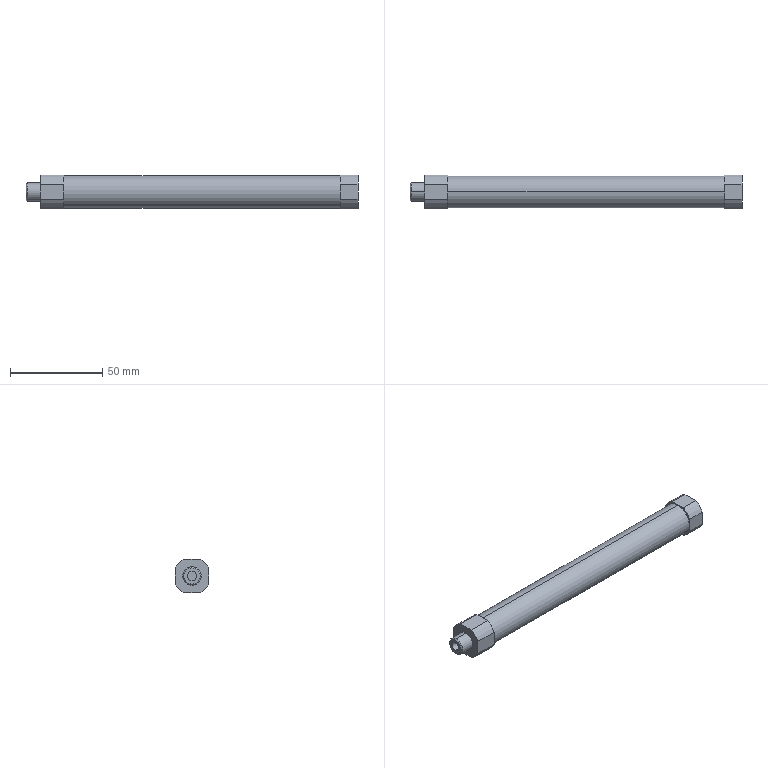Part | SolidWorks | features RefAxis 21, 3DProfileFeature 7, ICE 3, HoleWzd 2, RevCut 1, Revolution 1 | 1 solid | 45 faces | box 180 x 18.3 x 18.3 mm | volume 16108 mm3 | cylinder 20 | plane 15 | cone 10 | commonest cylinder face diameters 20 x8 4.134 x4 5 x2 10 x2 16 x2 17.4 x2
STEP:
#1=CARTESIAN_POINT('',(142.5,0.,-8.));
#2=VERTEX_POINT('',#1);
#3=CARTESIAN_POINT('',(142.5,0.,8.));
#4=VERTEX_POINT('',#3);
#5=CARTESIAN_POINT('',(142.5,0.,0.));
#6=DIRECTION('',(-1.,0.,0.));
#7=DIRECTION('',(0.,0.,1.));
#8=AXIS2_PLACEMENT_3D('',#5,#6,#7);
#9=CIRCLE('',#8,8.);
#10=EDGE_CURVE('',#2,#4,#9,.T.);
#11=ORIENTED_EDGE('',*,*,#10,.F.);
#12=CARTESIAN_POINT('',(12.5,0.,-8.));
#13=VERTEX_POINT('',#12);
#14=CARTESIAN_POINT('',(50.,0.,-8.));
#15=DIRECTION('',(-1.,0.,0.));
#16=VECTOR('',#15,1000.);
#17=LINE('',#14,#16);
#18=EDGE_CURVE('',#2,#13,#17,.T.);
#19=ORIENTED_EDGE('',*,*,#18,.T.);
#20=CARTESIAN_POINT('',(12.5,0.,8.));
#21=VERTEX_POINT('',#20);
#22=CARTESIAN_POINT('',(12.5,0.,0.));
#23=DIRECTION('',(-1.,0.,0.));
#24=DIRECTION('',(0.,0.,1.));
#25=AXIS2_PLACEMENT_3D('',#22,#23,#24);
#26=CIRCLE('',#25,8.);
#27=EDGE_CURVE('',#13,#21,#26,.T.);
#28=ORIENTED_EDGE('',*,*,#27,.T.);
#29=CARTESIAN_POINT('',(50.,0.,8.));
#30=DIRECTION('',(-1.,0.,0.));
#31=VECTOR('',#30,1000.);
#32=LINE('',#29,#31);
#33=EDGE_CURVE('',#4,#21,#32,.T.);
#34=ORIENTED_EDGE('',*,*,#33,.F.);
#35=EDGE_LOOP('',(#11,#19,#28,#34));
#36=FACE_OUTER_BOUND('',#35,.T.);
#37=CARTESIAN_POINT('',(50.,0.,0.));
#38=DIRECTION('',(-1.,0.,0.));
#39=DIRECTION('',(0.,0.,1.));
#40=AXIS2_PLACEMENT_3D('',#37,#38,#39);
#41=CYLINDRICAL_SURFACE('',#40,8.);
#42=ADVANCED_FACE('',(#36),#41,.F.);
#43=CARTESIAN_POINT('',(12.5,0.,-2.5));
#44=VERTEX_POINT('',#43);
#45=CARTESIAN_POINT('',(12.5,0.,2.5));
#46=VERTEX_POINT('',#45);
#47=CARTESIAN_POINT('',(12.5,0.,0.));
#48=DIRECTION('',(-1.,0.,0.));
#49=DIRECTION('',(0.,0.,1.));
#50=AXIS2_PLACEMENT_3D('',#47,#48,#49);
#51=CIRCLE('',#50,2.5);
#52=EDGE_CURVE('',#44,#46,#51,.T.);
#53=ORIENTED_EDGE('',*,*,#52,.F.);
#54=CARTESIAN_POINT('',(-8.,0.,-2.5));
#55=VERTEX_POINT('',#54);
#56=CARTESIAN_POINT('',(50.,0.,-2.5));
#57=DIRECTION('',(-1.,0.,0.));
#58=VECTOR('',#57,1000.);
#59=LINE('',#56,#58);
#60=EDGE_CURVE('',#44,#55,#59,.T.);
#61=ORIENTED_EDGE('',*,*,#60,.T.);
#62=CARTESIAN_POINT('',(-8.,0.,2.5));
#63=VERTEX_POINT('',#62);
#64=CARTESIAN_POINT('',(-8.,0.,0.));
#65=DIRECTION('',(-1.,0.,0.));
#66=DIRECTION('',(0.,0.,1.));
#67=AXIS2_PLACEMENT_3D('',#64,#65,#66);
#68=CIRCLE('',#67,2.5);
#69=EDGE_CURVE('',#55,#63,#68,.T.);
#70=ORIENTED_EDGE('',*,*,#69,.T.);
#71=CARTESIAN_POINT('',(50.,0.,2.5));
#72=DIRECTION('',(-1.,0.,0.));
#73=VECTOR('',#72,1000.);
#74=LINE('',#71,#73);
#75=EDGE_CURVE('',#46,#63,#74,.T.);
#76=ORIENTED_EDGE('',*,*,#75,.F.);
#77=EDGE_LOOP('',(#53,#61,#70,#76));
#78=FACE_OUTER_BOUND('',#77,.T.);
#79=CARTESIAN_POINT('',(50.,0.,0.));
#80=DIRECTION('',(-1.,0.,0.));
#81=DIRECTION('',(0.,0.,1.));
#82=AXIS2_PLACEMENT_3D('',#79,#80,#81);
#83=CYLINDRICAL_SURFACE('',#82,2.5);
#84=ADVANCED_FACE('',(#78),#83,.F.);
#85=CARTESIAN_POINT('',(167.,8.717,-2.067));
#86=VERTEX_POINT('',#85);
#87=CARTESIAN_POINT('',(167.,8.717,2.067));
#88=VERTEX_POINT('',#87);
#89=CARTESIAN_POINT('',(167.,8.717,0.));
#90=DIRECTION('',(0.,1.,0.));
#91=DIRECTION('',(0.,0.,1.));
#92=AXIS2_PLACEMENT_3D('',#89,#90,#91);
#93=CIRCLE('',#92,2.067);
#94=EDGE_CURVE('',#86,#88,#93,.T.);
#95=ORIENTED_EDGE('',*,*,#94,.F.);
#96=CARTESIAN_POINT('',(167.,9.15,-2.5));
#97=VERTEX_POINT('',#96);
#98=CARTESIAN_POINT('',(167.,9.15,-2.5));
#99=DIRECTION('',(0.,0.7071,-0.7071));
#100=VECTOR('',#99,1000.);
#101=LINE('',#98,#100);
#102=EDGE_CURVE('',#86,#97,#101,.T.);
#103=ORIENTED_EDGE('',*,*,#102,.T.);
#104=CARTESIAN_POINT('',(167.,9.15,2.5));
#105=VERTEX_POINT('',#104);
#106=CARTESIAN_POINT('',(167.,9.15,0.));
#107=DIRECTION('',(0.,1.,0.));
#108=DIRECTION('',(0.,0.,1.));
#109=AXIS2_PLACEMENT_3D('',#106,#107,#108);
#110=CIRCLE('',#109,2.5);
#111=EDGE_CURVE('',#97,#105,#110,.T.);
#112=ORIENTED_EDGE('',*,*,#111,.T.);
#113=CARTESIAN_POINT('',(167.,9.15,2.5));
#114=DIRECTION('',(0.,0.7071,0.7071));
#115=VECTOR('',#114,1000.);
#116=LINE('',#113,#115);
#117=EDGE_CURVE('',#88,#105,#116,.T.);
#118=ORIENTED_EDGE('',*,*,#117,.F.);
#119=EDGE_LOOP('',(#95,#103,#112,#118));
#120=FACE_OUTER_BOUND('',#119,.T.);
#121=CARTESIAN_POINT('',(167.,9.15,0.));
#122=DIRECTION('',(0.,1.,0.));
#123=DIRECTION('',(0.,0.,1.));
#124=AXIS2_PLACEMENT_3D('',#121,#122,#123);
#125=CONICAL_SURFACE('',#124,2.5,0.7854);
#126=ADVANCED_FACE('',(#120),#125,.F.);
#127=CARTESIAN_POINT('',(167.,4.15,-2.067));
#128=VERTEX_POINT('',#127);
#129=CARTESIAN_POINT('',(167.,4.15,2.067));
#130=VERTEX_POINT('',#129);
#131=CARTESIAN_POINT('',(167.,4.15,0.));
#132=DIRECTION('',(0.,1.,0.));
#133=DIRECTION('',(0.,0.,1.));
#134=AXIS2_PLACEMENT_3D('',#131,#132,#133);
#135=CIRCLE('',#134,2.067);
#136=EDGE_CURVE('',#128,#130,#135,.T.);
#137=ORIENTED_EDGE('',*,*,#136,.F.);
#138=CARTESIAN_POINT('',(167.,9.15,-2.067));
#139=DIRECTION('',(0.,1.,0.));
#140=VECTOR('',#139,1000.);
#141=LINE('',#138,#140);
#142=EDGE_CURVE('',#128,#86,#141,.T.);
#143=ORIENTED_EDGE('',*,*,#142,.T.);
#144=ORIENTED_EDGE('',*,*,#94,.T.);
#145=CARTESIAN_POINT('',(167.,9.15,2.067));
#146=DIRECTION('',(0.,1.,0.));
#147=VECTOR('',#146,1000.);
#148=LINE('',#145,#147);
#149=EDGE_CURVE('',#130,#88,#148,.T.);
#150=ORIENTED_EDGE('',*,*,#149,.F.);
#151=EDGE_LOOP('',(#137,#143,#144,#150));
#152=FACE_OUTER_BOUND('',#151,.T.);
#153=CARTESIAN_POINT('',(167.,9.15,0.));
#154=DIRECTION('',(0.,1.,0.));
#155=DIRECTION('',(0.,0.,1.));
#156=AXIS2_PLACEMENT_3D('',#153,#154,#155);
#157=CYLINDRICAL_SURFACE('',#156,2.067);
#158=ADVANCED_FACE('',(#152),#157,.F.);
#159=CARTESIAN_POINT('',(167.,2.957,0.));
#160=VERTEX_POINT('',#159);
#161=CARTESIAN_POINT('',(167.,4.15,2.067));
#162=DIRECTION('',(0.,0.5,0.866));
#163=VECTOR('',#162,1000.);
#164=LINE('',#161,#163);
#165=EDGE_CURVE('',#160,#130,#164,.T.);
#166=ORIENTED_EDGE('',*,*,#165,.F.);
#167=CARTESIAN_POINT('',(167.,4.15,-2.067));
#168=DIRECTION('',(0.,0.5,-0.866));
#169=VECTOR('',#168,1000.);
#170=LINE('',#167,#169);
#171=EDGE_CURVE('',#160,#128,#170,.T.);
#172=ORIENTED_EDGE('',*,*,#171,.T.);
#173=ORIENTED_EDGE('',*,*,#136,.T.);
#174=EDGE_LOOP('',(#166,#172,#173));
#175=FACE_OUTER_BOUND('',#174,.T.);
#176=CARTESIAN_POINT('',(167.,4.15,0.));
#177=DIRECTION('',(0.,1.,0.));
#178=DIRECTION('',(0.,0.,1.));
#179=AXIS2_PLACEMENT_3D('',#176,#177,#178);
#180=CONICAL_SURFACE('',#179,2.067,1.047);
#181=ADVANCED_FACE('',(#175),#180,.F.);
#182=CARTESIAN_POINT('',(8.,8.717,-2.067));
#183=VERTEX_POINT('',#182);
#184=CARTESIAN_POINT('',(8.,8.717,2.067));
#185=VERTEX_POINT('',#184);
#186=CARTESIAN_POINT('',(8.,8.717,0.));
#187=DIRECTION('',(0.,1.,0.));
#188=DIRECTION('',(0.,0.,1.));
#189=AXIS2_PLACEMENT_3D('',#186,#187,#188);
#190=CIRCLE('',#189,2.067);
#191=EDGE_CURVE('',#183,#185,#190,.T.);
#192=ORIENTED_EDGE('',*,*,#191,.F.);
#193=CARTESIAN_POINT('',(8.,9.15,-2.5));
#194=VERTEX_POINT('',#193);
#195=CARTESIAN_POINT('',(8.,9.15,-2.5));
#196=DIRECTION('',(0.,0.7071,-0.7071));
#197=VECTOR('',#196,1000.);
#198=LINE('',#195,#197);
#199=EDGE_CURVE('',#183,#194,#198,.T.);
#200=ORIENTED_EDGE('',*,*,#199,.T.);
#201=CARTESIAN_POINT('',(8.,9.15,2.5));
#202=VERTEX_POINT('',#201);
#203=CARTESIAN_POINT('',(8.,9.15,0.));
#204=DIRECTION('',(0.,1.,0.));
#205=DIRECTION('',(0.,0.,1.));
#206=AXIS2_PLACEMENT_3D('',#203,#204,#205);
#207=CIRCLE('',#206,2.5);
#208=EDGE_CURVE('',#194,#202,#207,.T.);
#209=ORIENTED_EDGE('',*,*,#208,.T.);
#210=CARTESIAN_POINT('',(8.,9.15,2.5));
#211=DIRECTION('',(0.,0.7071,0.7071));
#212=VECTOR('',#211,1000.);
#213=LINE('',#210,#212);
#214=EDGE_CURVE('',#185,#202,#213,.T.);
#215=ORIENTED_EDGE('',*,*,#214,.F.);
#216=EDGE_LOOP('',(#192,#200,#209,#215));
#217=FACE_OUTER_BOUND('',#216,.T.);
#218=CARTESIAN_POINT('',(8.,9.15,0.));
#219=DIRECTION('',(0.,1.,0.));
#220=DIRECTION('',(0.,0.,1.));
#221=AXIS2_PLACEMENT_3D('',#218,#219,#220);
#222=CONICAL_SURFACE('',#221,2.5,0.7854);
#223=ADVANCED_FACE('',(#217),#222,.F.);
#224=CARTESIAN_POINT('',(8.,4.15,-2.067));
#225=VERTEX_POINT('',#224);
#226=CARTESIAN_POINT('',(8.,4.15,2.067));
#227=VERTEX_POINT('',#226);
#228=CARTESIAN_POINT('',(8.,4.15,0.));
#229=DIRECTION('',(0.,1.,0.));
#230=DIRECTION('',(0.,0.,1.));
#231=AXIS2_PLACEMENT_3D('',#228,#229,#230);
#232=CIRCLE('',#231,2.067);
#233=EDGE_CURVE('',#225,#227,#232,.T.);
#234=ORIENTED_EDGE('',*,*,#233,.F.);
#235=CARTESIAN_POINT('',(8.,9.15,-2.067));
#236=DIRECTION('',(0.,1.,0.));
#237=VECTOR('',#236,1000.);
#238=LINE('',#235,#237);
#239=EDGE_CURVE('',#225,#183,#238,.T.);
#240=ORIENTED_EDGE('',*,*,#239,.T.);
#241=ORIENTED_EDGE('',*,*,#191,.T.);
#242=CARTESIAN_POINT('',(8.,9.15,2.067));
#243=DIRECTION('',(0.,1.,0.));
#244=VECTOR('',#243,1000.);
#245=LINE('',#242,#244);
#246=EDGE_CURVE('',#227,#185,#245,.T.);
#247=ORIENTED_EDGE('',*,*,#246,.F.);
#248=EDGE_LOOP('',(#234,#240,#241,#247));
#249=FACE_OUTER_BOUND('',#248,.T.);
#250=CARTESIAN_POINT('',(8.,9.15,0.));
#251=DIRECTION('',(0.,1.,0.));
#252=DIRECTION('',(0.,0.,1.));
#253=AXIS2_PLACEMENT_3D('',#250,#251,#252);
#254=CYLINDRICAL_SURFACE('',#253,2.067);
#255=ADVANCED_FACE('',(#249),#254,.F.);
#256=CARTESIAN_POINT('',(8.,2.957,0.));
#257=VERTEX_POINT('',#256);
#258=CARTESIAN_POINT('',(8.,4.15,2.067));
#259=DIRECTION('',(0.,0.5,0.866));
#260=VECTOR('',#259,1000.);
#261=LINE('',#258,#260);
#262=EDGE_CURVE('',#257,#227,#261,.T.);
#263=ORIENTED_EDGE('',*,*,#262,.F.);
#264=CARTESIAN_POINT('',(8.,4.15,-2.067));
#265=DIRECTION('',(0.,0.5,-0.866));
#266=VECTOR('',#265,1000.);
#267=LINE('',#264,#266);
#268=EDGE_CURVE('',#257,#225,#267,.T.);
#269=ORIENTED_EDGE('',*,*,#268,.T.);
#270=ORIENTED_EDGE('',*,*,#233,.T.);
#271=EDGE_LOOP('',(#263,#269,#270));
#272=FACE_OUTER_BOUND('',#271,.T.);
#273=CARTESIAN_POINT('',(8.,4.15,0.));
#274=DIRECTION('',(0.,1.,0.));
#275=DIRECTION('',(0.,0.,1.));
#276=AXIS2_PLACEMENT_3D('',#273,#274,#275);
#277=CONICAL_SURFACE('',#276,2.067,1.047);
#278=ADVANCED_FACE('',(#272),#277,.F.);
#279=CARTESIAN_POINT('',(162.5,0.,-8.7));
#280=VERTEX_POINT('',#279);
#281=CARTESIAN_POINT('',(162.5,0.,8.7));
#282=VERTEX_POINT('',#281);
#283=CARTESIAN_POINT('',(162.5,0.,0.));
#284=DIRECTION('',(1.,0.,0.));
#285=DIRECTION('',(0.,0.,-1.));
#286=AXIS2_PLACEMENT_3D('',#283,#284,#285);
#287=CIRCLE('',#286,8.7);
#288=EDGE_CURVE('',#280,#282,#287,.T.);
#289=ORIENTED_EDGE('',*,*,#288,.F.);
#290=CARTESIAN_POINT('',(12.5,0.,-8.7));
#291=VERTEX_POINT('',#290);
#292=CARTESIAN_POINT('',(162.5,0.,-8.7));
#293=DIRECTION('',(-1.,0.,0.));
#294=VECTOR('',#293,1000.);
#295=LINE('',#292,#294);
#296=EDGE_CURVE('',#280,#291,#295,.T.);
#297=ORIENTED_EDGE('',*,*,#296,.T.);
#298=CARTESIAN_POINT('',(12.5,0.,8.7));
#299=VERTEX_POINT('',#298);
#300=CARTESIAN_POINT('',(12.5,0.,0.));
#301=DIRECTION('',(1.,0.,0.));
#302=DIRECTION('',(0.,0.,-1.));
#303=AXIS2_PLACEMENT_3D('',#300,#301,#302);
#304=CIRCLE('',#303,8.7);
#305=EDGE_CURVE('',#291,#299,#304,.T.);
#306=ORIENTED_EDGE('',*,*,#305,.T.);
#307=CARTESIAN_POINT('',(162.5,0.,8.7));
#308=DIRECTION('',(-1.,0.,0.));
#309=VECTOR('',#308,1000.);
#310=LINE('',#307,#309);
#311=EDGE_CURVE('',#282,#299,#310,.T.);
#312=ORIENTED_EDGE('',*,*,#311,.F.);
#313=EDGE_LOOP('',(#289,#297,#306,#312));
#314=FACE_OUTER_BOUND('',#313,.T.);
#315=CARTESIAN_POINT('',(162.5,0.,0.));
#316=DIRECTION('',(-1.,0.,0.));
#317=DIRECTION('',(0.,0.,1.));
#318=AXIS2_PLACEMENT_3D('',#315,#316,#317);
#319=CYLINDRICAL_SURFACE('',#318,8.7);
#320=ADVANCED_FACE('',(#314),#319,.T.);
#321=CARTESIAN_POINT('',(0.,0.,-5.));
#322=VERTEX_POINT('',#321);
#323=CARTESIAN_POINT('',(0.,0.,5.));
#324=VERTEX_POINT('',#323);
#325=CARTESIAN_POINT('',(0.,0.,0.));
#326=DIRECTION('',(1.,0.,0.));
#327=DIRECTION('',(0.,0.,-1.));
#328=AXIS2_PLACEMENT_3D('',#325,#326,#327);
#329=CIRCLE('',#328,5.);
#330=EDGE_CURVE('',#322,#324,#329,.T.);
#331=ORIENTED_EDGE('',*,*,#330,.F.);
#332=CARTESIAN_POINT('',(-7.386,0.,-5.));
#333=VERTEX_POINT('',#332);
#334=CARTESIAN_POINT('',(0.,0.,-5.));
#335=DIRECTION('',(-1.,0.,0.));
#336=VECTOR('',#335,1000.);
#337=LINE('',#334,#336);
#338=EDGE_CURVE('',#322,#333,#337,.T.);
#339=ORIENTED_EDGE('',*,*,#338,.T.);
#340=CARTESIAN_POINT('',(-7.386,0.,5.));
#341=VERTEX_POINT('',#340);
#342=CARTESIAN_POINT('',(-7.386,0.,0.));
#343=DIRECTION('',(-1.,0.,0.));
#344=DIRECTION('',(0.,0.,1.));
#345=AXIS2_PLACEMENT_3D('',#342,#343,#344);
#346=CIRCLE('',#345,5.);
#347=EDGE_CURVE('',#341,#333,#346,.T.);
#348=ORIENTED_EDGE('',*,*,#347,.F.);
#349=CARTESIAN_POINT('',(0.,0.,5.));
#350=DIRECTION('',(-1.,0.,0.));
#351=VECTOR('',#350,1000.);
#352=LINE('',#349,#351);
#353=EDGE_CURVE('',#324,#341,#352,.T.);
#354=ORIENTED_EDGE('',*,*,#353,.F.);
#355=EDGE_LOOP('',(#331,#339,#348,#354));
#356=FACE_OUTER_BOUND('',#355,.T.);
#357=CARTESIAN_POINT('',(0.,0.,0.));
#358=DIRECTION('',(-1.,0.,0.));
#359=DIRECTION('',(0.,0.,1.));
#360=AXIS2_PLACEMENT_3D('',#357,#358,#359);
#361=CYLINDRICAL_SURFACE('',#360,5.);
#362=ADVANCED_FACE('',(#356),#361,.T.);
#363=CARTESIAN_POINT('',(-8.,0.,4.386));
#364=VERTEX_POINT('',#363);
#365=CARTESIAN_POINT('',(-8.,0.,-4.386));
#366=VERTEX_POINT('',#365);
#367=CARTESIAN_POINT('',(-8.,0.,0.));
#368=DIRECTION('',(-1.,0.,0.));
#369=DIRECTION('',(0.,0.,1.));
#370=AXIS2_PLACEMENT_3D('',#367,#368,#369);
#371=CIRCLE('',#370,4.386);
#372=EDGE_CURVE('',#364,#366,#371,.T.);
#373=ORIENTED_EDGE('',*,*,#372,.F.);
#374=CARTESIAN_POINT('',(-7.386,0.,5.));
#375=DIRECTION('',(0.7071,0.,0.7071));
#376=VECTOR('',#375,1000.);
#377=LINE('',#374,#376);
#378=EDGE_CURVE('',#364,#341,#377,.T.);
#379=ORIENTED_EDGE('',*,*,#378,.T.);
#380=ORIENTED_EDGE('',*,*,#347,.T.);
#381=CARTESIAN_POINT('',(-7.386,0.,-5.));
#382=DIRECTION('',(0.7071,0.,-0.7071));
#383=VECTOR('',#382,1000.);
#384=LINE('',#381,#383);
#385=EDGE_CURVE('',#366,#333,#384,.T.);
#386=ORIENTED_EDGE('',*,*,#385,.F.);
#387=EDGE_LOOP('',(#373,#379,#380,#386));
#388=FACE_OUTER_BOUND('',#387,.T.);
#389=CARTESIAN_POINT('',(-7.386,0.,0.));
#390=DIRECTION('',(1.,0.,0.));
#391=DIRECTION('',(0.,0.,-1.));
#392=AXIS2_PLACEMENT_3D('',#389,#390,#391);
#393=CONICAL_SURFACE('',#392,5.,0.7854);
#394=ADVANCED_FACE('',(#388),#393,.T.);
#395=CARTESIAN_POINT('',(-8.,0.,0.));
#396=DIRECTION('',(-1.,0.,0.));
#397=DIRECTION('',(0.,0.,1.));
#398=AXIS2_PLACEMENT_3D('',#395,#396,#397);
#399=CIRCLE('',#398,4.386);
#400=EDGE_CURVE('',#366,#364,#399,.T.);
#401=ORIENTED_EDGE('',*,*,#400,.T.);
#402=ORIENTED_EDGE('',*,*,#372,.T.);
#403=EDGE_LOOP('',(#401,#402));
#404=FACE_OUTER_BOUND('',#403,.T.);
#405=CARTESIAN_POINT('',(-8.,0.,0.));
#406=DIRECTION('',(-1.,0.,0.));
#407=DIRECTION('',(0.,0.,1.));
#408=AXIS2_PLACEMENT_3D('',#405,#406,#407);
#409=CIRCLE('',#408,2.5);
#410=EDGE_CURVE('',#63,#55,#409,.T.);
#411=ORIENTED_EDGE('',*,*,#410,.F.);
#412=ORIENTED_EDGE('',*,*,#69,.F.);
#413=EDGE_LOOP('',(#411,#412));
#414=FACE_BOUND('',#413,.T.);
#415=CARTESIAN_POINT('',(-8.,0.,0.));
#416=DIRECTION('',(1.,0.,0.));
#417=DIRECTION('',(0.,0.,-1.));
#418=AXIS2_PLACEMENT_3D('',#415,#416,#417);
#419=PLANE('',#418);
#420=ADVANCED_FACE('',(#404,#414),#419,.F.);
#421=CARTESIAN_POINT('',(12.5,-4.035,9.15));
#422=VERTEX_POINT('',#421);
#423=CARTESIAN_POINT('',(12.5,-9.15,4.035));
#424=VERTEX_POINT('',#423);
#425=CARTESIAN_POINT('',(12.5,0.,0.));
#426=DIRECTION('',(1.,0.,0.));
#427=DIRECTION('',(0.,0.,-1.));
#428=AXIS2_PLACEMENT_3D('',#425,#426,#427);
#429=CIRCLE('',#428,10.);
#430=EDGE_CURVE('',#422,#424,#429,.T.);
#431=ORIENTED_EDGE('',*,*,#430,.T.);
#432=CARTESIAN_POINT('',(12.5,-9.15,-4.035));
#433=VERTEX_POINT('',#432);
#434=CARTESIAN_POINT('',(12.5,-9.15,4.035));
#435=DIRECTION('',(0.,0.,-1.));
#436=VECTOR('',#435,1000.);
#437=LINE('',#434,#436);
#438=EDGE_CURVE('',#424,#433,#437,.T.);
#439=ORIENTED_EDGE('',*,*,#438,.T.);
#440=CARTESIAN_POINT('',(12.5,-4.035,-9.15));
#441=VERTEX_POINT('',#440);
#442=CARTESIAN_POINT('',(12.5,0.,0.));
#443=DIRECTION('',(1.,0.,0.));
#444=DIRECTION('',(0.,0.,-1.));
#445=AXIS2_PLACEMENT_3D('',#442,#443,#444);
#446=CIRCLE('',#445,10.);
#447=EDGE_CURVE('',#433,#441,#446,.T.);
#448=ORIENTED_EDGE('',*,*,#447,.T.);
#449=CARTESIAN_POINT('',(12.5,4.035,-9.15));
#450=VERTEX_POINT('',#449);
#451=CARTESIAN_POINT('',(12.5,-4.035,-9.15));
#452=DIRECTION('',(0.,1.,0.));
#453=VECTOR('',#452,1000.);
#454=LINE('',#451,#453);
#455=EDGE_CURVE('',#441,#450,#454,.T.);
#456=ORIENTED_EDGE('',*,*,#455,.T.);
#457=CARTESIAN_POINT('',(12.5,9.15,-4.035));
#458=VERTEX_POINT('',#457);
#459=CARTESIAN_POINT('',(12.5,0.,0.));
#460=DIRECTION('',(1.,0.,0.));
#461=DIRECTION('',(0.,0.,-1.));
#462=AXIS2_PLACEMENT_3D('',#459,#460,#461);
#463=CIRCLE('',#462,10.);
#464=EDGE_CURVE('',#450,#458,#463,.T.);
#465=ORIENTED_EDGE('',*,*,#464,.T.);
#466=CARTESIAN_POINT('',(12.5,9.15,4.035));
#467=VERTEX_POINT('',#466);
#468=CARTESIAN_POINT('',(12.5,9.15,-4.035));
#469=DIRECTION('',(0.,0.,1.));
#470=VECTOR('',#469,1000.);
#471=LINE('',#468,#470);
#472=EDGE_CURVE('',#458,#467,#471,.T.);
#473=ORIENTED_EDGE('',*,*,#472,.T.);
#474=CARTESIAN_POINT('',(12.5,4.035,9.15));
#475=VERTEX_POINT('',#474);
#476=CARTESIAN_POINT('',(12.5,0.,0.));
#477=DIRECTION('',(1.,0.,0.));
#478=DIRECTION('',(0.,0.,-1.));
#479=AXIS2_PLACEMENT_3D('',#476,#477,#478);
#480=CIRCLE('',#479,10.);
#481=EDGE_CURVE('',#467,#475,#480,.T.);
#482=ORIENTED_EDGE('',*,*,#481,.T.);
#483=CARTESIAN_POINT('',(12.5,4.035,9.15));
#484=DIRECTION('',(0.,-1.,0.));
#485=VECTOR('',#484,1000.);
#486=LINE('',#483,#485);
#487=EDGE_CURVE('',#475,#422,#486,.T.);
#488=ORIENTED_EDGE('',*,*,#487,.T.);
#489=EDGE_LOOP('',(#431,#439,#448,#456,#465,#473,#482,#488));
#490=FACE_OUTER_BOUND('',#489,.T.);
#491=CARTESIAN_POINT('',(12.5,0.,0.));
#492=DIRECTION('',(1.,0.,0.));
#493=DIRECTION('',(0.,0.,-1.));
#494=AXIS2_PLACEMENT_3D('',#491,#492,#493);
#495=CIRCLE('',#494,8.7);
#496=EDGE_CURVE('',#299,#291,#495,.T.);
#497=ORIENTED_EDGE('',*,*,#496,.F.);
#498=ORIENTED_EDGE('',*,*,#305,.F.);
#499=EDGE_LOOP('',(#497,#498));
#500=FACE_BOUND('',#499,.T.);
#501=CARTESIAN_POINT('',(12.5,0.,0.));
#502=DIRECTION('',(1.,0.,0.));
#503=DIRECTION('',(0.,0.,-1.));
#504=AXIS2_PLACEMENT_3D('',#501,#502,#503);
#505=PLANE('',#504);
#506=ADVANCED_FACE('',(#490,#500),#505,.T.);
#507=ORIENTED_EDGE('',*,*,#378,.F.);
#508=ORIENTED_EDGE('',*,*,#400,.F.);
#509=ORIENTED_EDGE('',*,*,#385,.T.);
#510=CARTESIAN_POINT('',(-7.386,0.,0.));
#511=DIRECTION('',(-1.,0.,0.));
#512=DIRECTION('',(0.,0.,1.));
#513=AXIS2_PLACEMENT_3D('',#510,#511,#512);
#514=CIRCLE('',#513,5.);
#515=EDGE_CURVE('',#333,#341,#514,.T.);
#516=ORIENTED_EDGE('',*,*,#515,.T.);
#517=EDGE_LOOP('',(#507,#508,#509,#516));
#518=FACE_OUTER_BOUND('',#517,.T.);
#519=CARTESIAN_POINT('',(-7.386,0.,0.));
#520=DIRECTION('',(1.,0.,0.));
#521=DIRECTION('',(0.,0.,-1.));
#522=AXIS2_PLACEMENT_3D('',#519,#520,#521);
#523=CONICAL_SURFACE('',#522,5.,0.7854);
#524=ADVANCED_FACE('',(#518),#523,.T.);
#525=ORIENTED_EDGE('',*,*,#338,.F.);
#526=CARTESIAN_POINT('',(0.,0.,0.));
#527=DIRECTION('',(1.,0.,0.));
#528=DIRECTION('',(0.,0.,-1.));
#529=AXIS2_PLACEMENT_3D('',#526,#527,#528);
#530=CIRCLE('',#529,5.);
#531=EDGE_CURVE('',#324,#322,#530,.T.);
#532=ORIENTED_EDGE('',*,*,#531,.F.);
#533=ORIENTED_EDGE('',*,*,#353,.T.);
#534=ORIENTED_EDGE('',*,*,#515,.F.);
#535=EDGE_LOOP('',(#525,#532,#533,#534));
#536=FACE_OUTER_BOUND('',#535,.T.);
#537=CARTESIAN_POINT('',(0.,0.,0.));
#538=DIRECTION('',(-1.,0.,0.));
#539=DIRECTION('',(0.,0.,1.));
#540=AXIS2_PLACEMENT_3D('',#537,#538,#539);
#541=CYLINDRICAL_SURFACE('',#540,5.);
#542=ADVANCED_FACE('',(#536),#541,.T.);
#543=CARTESIAN_POINT('',(0.,-4.035,9.15));
#544=VERTEX_POINT('',#543);
#545=CARTESIAN_POINT('',(0.,-9.15,4.035));
#546=VERTEX_POINT('',#545);
#547=CARTESIAN_POINT('',(0.,0.,0.));
#548=DIRECTION('',(1.,0.,0.));
#549=DIRECTION('',(0.,0.,-1.));
#550=AXIS2_PLACEMENT_3D('',#547,#548,#549);
#551=CIRCLE('',#550,10.);
#552=EDGE_CURVE('',#544,#546,#551,.T.);
#553=ORIENTED_EDGE('',*,*,#552,.F.);
#554=CARTESIAN_POINT('',(0.,4.035,9.15));
#555=VERTEX_POINT('',#554);
#556=CARTESIAN_POINT('',(0.,4.035,9.15));
#557=DIRECTION('',(0.,-1.,0.));
#558=VECTOR('',#557,1000.);
#559=LINE('',#556,#558);
#560=EDGE_CURVE('',#555,#544,#559,.T.);
#561=ORIENTED_EDGE('',*,*,#560,.F.);
#562=CARTESIAN_POINT('',(0.,9.15,4.035));
#563=VERTEX_POINT('',#562);
#564=CARTESIAN_POINT('',(0.,0.,0.));
#565=DIRECTION('',(1.,0.,0.));
#566=DIRECTION('',(0.,0.,-1.));
#567=AXIS2_PLACEMENT_3D('',#564,#565,#566);
#568=CIRCLE('',#567,10.);
#569=EDGE_CURVE('',#563,#555,#568,.T.);
#570=ORIENTED_EDGE('',*,*,#569,.F.);
#571=CARTESIAN_POINT('',(0.,9.15,-4.035));
#572=VERTEX_POINT('',#571);
#573=CARTESIAN_POINT('',(0.,9.15,-4.035));
#574=DIRECTION('',(0.,0.,1.));
#575=VECTOR('',#574,1000.);
#576=LINE('',#573,#575);
#577=EDGE_CURVE('',#572,#563,#576,.T.);
#578=ORIENTED_EDGE('',*,*,#577,.F.);
#579=CARTESIAN_POINT('',(0.,4.035,-9.15));
#580=VERTEX_POINT('',#579);
#581=CARTESIAN_POINT('',(0.,0.,0.));
#582=DIRECTION('',(1.,0.,0.));
#583=DIRECTION('',(0.,0.,-1.));
#584=AXIS2_PLACEMENT_3D('',#581,#582,#583);
#585=CIRCLE('',#584,10.);
#586=EDGE_CURVE('',#580,#572,#585,.T.);
#587=ORIENTED_EDGE('',*,*,#586,.F.);
#588=CARTESIAN_POINT('',(0.,-4.035,-9.15));
#589=VERTEX_POINT('',#588);
#590=CARTESIAN_POINT('',(0.,-4.035,-9.15));
#591=DIRECTION('',(0.,1.,0.));
#592=VECTOR('',#591,1000.);
#593=LINE('',#590,#592);
#594=EDGE_CURVE('',#589,#580,#593,.T.);
#595=ORIENTED_EDGE('',*,*,#594,.F.);
#596=CARTESIAN_POINT('',(0.,-9.15,-4.035));
#597=VERTEX_POINT('',#596);
#598=CARTESIAN_POINT('',(0.,0.,0.));
#599=DIRECTION('',(1.,0.,0.));
#600=DIRECTION('',(0.,0.,-1.));
#601=AXIS2_PLACEMENT_3D('',#598,#599,#600);
#602=CIRCLE('',#601,10.);
#603=EDGE_CURVE('',#597,#589,#602,.T.);
#604=ORIENTED_EDGE('',*,*,#603,.F.);
#605=CARTESIAN_POINT('',(0.,-9.15,4.035));
#606=DIRECTION('',(0.,0.,-1.));
#607=VECTOR('',#606,1000.);
#608=LINE('',#605,#607);
#609=EDGE_CURVE('',#546,#597,#608,.T.);
#610=ORIENTED_EDGE('',*,*,#609,.F.);
#611=EDGE_LOOP('',(#553,#561,#570,#578,#587,#595,#604,#610));
#612=FACE_OUTER_BOUND('',#611,.T.);
#613=ORIENTED_EDGE('',*,*,#531,.T.);
#614=ORIENTED_EDGE('',*,*,#330,.T.);
#615=EDGE_LOOP('',(#613,#614));
#616=FACE_BOUND('',#615,.T.);
#617=CARTESIAN_POINT('',(0.,0.,0.));
#618=DIRECTION('',(1.,0.,0.));
#619=DIRECTION('',(0.,0.,-1.));
#620=AXIS2_PLACEMENT_3D('',#617,#618,#619);
#621=PLANE('',#620);
#622=ADVANCED_FACE('',(#612,#616),#621,.F.);
#623=ORIENTED_EDGE('',*,*,#552,.T.);
#624=CARTESIAN_POINT('',(12.5,-9.15,4.035));
#625=DIRECTION('',(-1.,0.,0.));
#626=VECTOR('',#625,1000.);
#627=LINE('',#624,#626);
#628=EDGE_CURVE('',#424,#546,#627,.T.);
#629=ORIENTED_EDGE('',*,*,#628,.F.);
#630=ORIENTED_EDGE('',*,*,#430,.F.);
#631=CARTESIAN_POINT('',(12.5,-4.035,9.15));
#632=DIRECTION('',(-1.,0.,0.));
#633=VECTOR('',#632,1000.);
#634=LINE('',#631,#633);
#635=EDGE_CURVE('',#422,#544,#634,.T.);
#636=ORIENTED_EDGE('',*,*,#635,.T.);
#637=EDGE_LOOP('',(#623,#629,#630,#636));
#638=FACE_OUTER_BOUND('',#637,.T.);
#639=CARTESIAN_POINT('',(12.5,0.,0.));
#640=DIRECTION('',(-1.,0.,0.));
#641=DIRECTION('',(0.,0.,1.));
#642=AXIS2_PLACEMENT_3D('',#639,#640,#641);
#643=CYLINDRICAL_SURFACE('',#642,10.);
#644=ADVANCED_FACE('',(#638),#643,.T.);
#645=ORIENTED_EDGE('',*,*,#609,.T.);
#646=CARTESIAN_POINT('',(12.5,-9.15,-4.035));
#647=DIRECTION('',(-1.,0.,0.));
#648=VECTOR('',#647,1000.);
#649=LINE('',#646,#648);
#650=EDGE_CURVE('',#433,#597,#649,.T.);
#651=ORIENTED_EDGE('',*,*,#650,.F.);
#652=ORIENTED_EDGE('',*,*,#438,.F.);
#653=ORIENTED_EDGE('',*,*,#628,.T.);
#654=EDGE_LOOP('',(#645,#651,#652,#653));
#655=FACE_OUTER_BOUND('',#654,.T.);
#656=CARTESIAN_POINT('',(12.5,-9.15,4.035));
#657=DIRECTION('',(0.,1.,0.));
#658=DIRECTION('',(0.,0.,1.));
#659=AXIS2_PLACEMENT_3D('',#656,#657,#658);
#660=PLANE('',#659);
#661=ADVANCED_FACE('',(#655),#660,.F.);
#662=ORIENTED_EDGE('',*,*,#603,.T.);
#663=CARTESIAN_POINT('',(12.5,-4.035,-9.15));
#664=DIRECTION('',(-1.,0.,0.));
#665=VECTOR('',#664,1000.);
#666=LINE('',#663,#665);
#667=EDGE_CURVE('',#441,#589,#666,.T.);
#668=ORIENTED_EDGE('',*,*,#667,.F.);
#669=ORIENTED_EDGE('',*,*,#447,.F.);
#670=ORIENTED_EDGE('',*,*,#650,.T.);
#671=EDGE_LOOP('',(#662,#668,#669,#670));
#672=FACE_OUTER_BOUND('',#671,.T.);
#673=CARTESIAN_POINT('',(12.5,0.,0.));
#674=DIRECTION('',(-1.,0.,0.));
#675=DIRECTION('',(0.,0.,1.));
#676=AXIS2_PLACEMENT_3D('',#673,#674,#675);
#677=CYLINDRICAL_SURFACE('',#676,10.);
#678=ADVANCED_FACE('',(#672),#677,.T.);
#679=ORIENTED_EDGE('',*,*,#594,.T.);
#680=CARTESIAN_POINT('',(12.5,4.035,-9.15));
#681=DIRECTION('',(-1.,0.,0.));
#682=VECTOR('',#681,1000.);
#683=LINE('',#680,#682);
#684=EDGE_CURVE('',#450,#580,#683,.T.);
#685=ORIENTED_EDGE('',*,*,#684,.F.);
#686=ORIENTED_EDGE('',*,*,#455,.F.);
#687=ORIENTED_EDGE('',*,*,#667,.T.);
#688=EDGE_LOOP('',(#679,#685,#686,#687));
#689=FACE_OUTER_BOUND('',#688,.T.);
#690=CARTESIAN_POINT('',(12.5,-4.035,-9.15));
#691=DIRECTION('',(0.,0.,1.));
#692=DIRECTION('',(1.,0.,0.));
#693=AXIS2_PLACEMENT_3D('',#690,#691,#692);
#694=PLANE('',#693);
#695=ADVANCED_FACE('',(#689),#694,.F.);
#696=ORIENTED_EDGE('',*,*,#586,.T.);
#697=CARTESIAN_POINT('',(12.5,9.15,-4.035));
#698=DIRECTION('',(-1.,0.,0.));
#699=VECTOR('',#698,1000.);
#700=LINE('',#697,#699);
#701=EDGE_CURVE('',#458,#572,#700,.T.);
#702=ORIENTED_EDGE('',*,*,#701,.F.);
#703=ORIENTED_EDGE('',*,*,#464,.F.);
#704=ORIENTED_EDGE('',*,*,#684,.T.);
#705=EDGE_LOOP('',(#696,#702,#703,#704));
#706=FACE_OUTER_BOUND('',#705,.T.);
#707=CARTESIAN_POINT('',(12.5,0.,0.));
#708=DIRECTION('',(-1.,0.,0.));
#709=DIRECTION('',(0.,0.,1.));
#710=AXIS2_PLACEMENT_3D('',#707,#708,#709);
#711=CYLINDRICAL_SURFACE('',#710,10.);
#712=ADVANCED_FACE('',(#706),#711,.T.);
#713=CARTESIAN_POINT('',(8.,9.15,0.));
#714=DIRECTION('',(0.,1.,0.));
#715=DIRECTION('',(0.,0.,1.));
#716=AXIS2_PLACEMENT_3D('',#713,#714,#715);
#717=CIRCLE('',#716,2.5);
#718=EDGE_CURVE('',#202,#194,#717,.T.);
#719=ORIENTED_EDGE('',*,*,#718,.F.);
#720=ORIENTED_EDGE('',*,*,#208,.F.);
#721=EDGE_LOOP('',(#719,#720));
#722=FACE_BOUND('',#721,.T.);
#723=ORIENTED_EDGE('',*,*,#577,.T.);
#724=CARTESIAN_POINT('',(12.5,9.15,4.035));
#725=DIRECTION('',(-1.,0.,0.));
#726=VECTOR('',#725,1000.);
#727=LINE('',#724,#726);
#728=EDGE_CURVE('',#467,#563,#727,.T.);
#729=ORIENTED_EDGE('',*,*,#728,.F.);
#730=ORIENTED_EDGE('',*,*,#472,.F.);
#731=ORIENTED_EDGE('',*,*,#701,.T.);
#732=EDGE_LOOP('',(#723,#729,#730,#731));
#733=FACE_OUTER_BOUND('',#732,.T.);
#734=CARTESIAN_POINT('',(12.5,9.15,-4.035));
#735=DIRECTION('',(0.,-1.,0.));
#736=DIRECTION('',(0.,0.,-1.));
#737=AXIS2_PLACEMENT_3D('',#734,#735,#736);
#738=PLANE('',#737);
#739=ADVANCED_FACE('',(#722,#733),#738,.F.);
#740=ORIENTED_EDGE('',*,*,#569,.T.);
#741=CARTESIAN_POINT('',(12.5,4.035,9.15));
#742=DIRECTION('',(-1.,0.,0.));
#743=VECTOR('',#742,1000.);
#744=LINE('',#741,#743);
#745=EDGE_CURVE('',#475,#555,#744,.T.);
#746=ORIENTED_EDGE('',*,*,#745,.F.);
#747=ORIENTED_EDGE('',*,*,#481,.F.);
#748=ORIENTED_EDGE('',*,*,#728,.T.);
#749=EDGE_LOOP('',(#740,#746,#747,#748));
#750=FACE_OUTER_BOUND('',#749,.T.);
#751=CARTESIAN_POINT('',(12.5,0.,0.));
#752=DIRECTION('',(-1.,0.,0.));
#753=DIRECTION('',(0.,0.,1.));
#754=AXIS2_PLACEMENT_3D('',#751,#752,#753);
#755=CYLINDRICAL_SURFACE('',#754,10.);
#756=ADVANCED_FACE('',(#750),#755,.T.);
#757=ORIENTED_EDGE('',*,*,#560,.T.);
#758=ORIENTED_EDGE('',*,*,#635,.F.);
#759=ORIENTED_EDGE('',*,*,#487,.F.);
#760=ORIENTED_EDGE('',*,*,#745,.T.);
#761=EDGE_LOOP('',(#757,#758,#759,#760));
#762=FACE_OUTER_BOUND('',#761,.T.);
#763=CARTESIAN_POINT('',(12.5,4.035,9.15));
#764=DIRECTION('',(0.,0.,-1.));
#765=DIRECTION('',(-1.,0.,0.));
#766=AXIS2_PLACEMENT_3D('',#763,#764,#765);
#767=PLANE('',#766);
#768=ADVANCED_FACE('',(#762),#767,.F.);
#769=ORIENTED_EDGE('',*,*,#296,.F.);
#770=CARTESIAN_POINT('',(162.5,0.,0.));
#771=DIRECTION('',(1.,0.,0.));
#772=DIRECTION('',(0.,0.,-1.));
#773=AXIS2_PLACEMENT_3D('',#770,#771,#772);
#774=CIRCLE('',#773,8.7);
#775=EDGE_CURVE('',#282,#280,#774,.T.);
#776=ORIENTED_EDGE('',*,*,#775,.F.);
#777=ORIENTED_EDGE('',*,*,#311,.T.);
#778=ORIENTED_EDGE('',*,*,#496,.T.);
#779=EDGE_LOOP('',(#769,#776,#777,#778));
#780=FACE_OUTER_BOUND('',#779,.T.);
#781=CARTESIAN_POINT('',(162.5,0.,0.));
#782=DIRECTION('',(-1.,0.,0.));
#783=DIRECTION('',(0.,0.,1.));
#784=AXIS2_PLACEMENT_3D('',#781,#782,#783);
#785=CYLINDRICAL_SURFACE('',#784,8.7);
#786=ADVANCED_FACE('',(#780),#785,.T.);
#787=CARTESIAN_POINT('',(162.5,-4.035,9.15));
#788=VERTEX_POINT('',#787);
#789=CARTESIAN_POINT('',(162.5,-9.15,4.035));
#790=VERTEX_POINT('',#789);
#791=CARTESIAN_POINT('',(162.5,0.,0.));
#792=DIRECTION('',(1.,0.,0.));
#793=DIRECTION('',(0.,0.,-1.));
#794=AXIS2_PLACEMENT_3D('',#791,#792,#793);
#795=CIRCLE('',#794,10.);
#796=EDGE_CURVE('',#788,#790,#795,.T.);
#797=ORIENTED_EDGE('',*,*,#796,.F.);
#798=CARTESIAN_POINT('',(162.5,4.035,9.15));
#799=VERTEX_POINT('',#798);
#800=CARTESIAN_POINT('',(162.5,4.035,9.15));
#801=DIRECTION('',(0.,-1.,0.));
#802=VECTOR('',#801,1000.);
#803=LINE('',#800,#802);
#804=EDGE_CURVE('',#799,#788,#803,.T.);
#805=ORIENTED_EDGE('',*,*,#804,.F.);
#806=CARTESIAN_POINT('',(162.5,9.15,4.035));
#807=VERTEX_POINT('',#806);
#808=CARTESIAN_POINT('',(162.5,0.,0.));
#809=DIRECTION('',(1.,0.,0.));
#810=DIRECTION('',(0.,0.,-1.));
#811=AXIS2_PLACEMENT_3D('',#808,#809,#810);
#812=CIRCLE('',#811,10.);
#813=EDGE_CURVE('',#807,#799,#812,.T.);
#814=ORIENTED_EDGE('',*,*,#813,.F.);
#815=CARTESIAN_POINT('',(162.5,9.15,-4.035));
#816=VERTEX_POINT('',#815);
#817=CARTESIAN_POINT('',(162.5,9.15,-4.035));
#818=DIRECTION('',(0.,0.,1.));
#819=VECTOR('',#818,1000.);
#820=LINE('',#817,#819);
#821=EDGE_CURVE('',#816,#807,#820,.T.);
#822=ORIENTED_EDGE('',*,*,#821,.F.);
#823=CARTESIAN_POINT('',(162.5,4.035,-9.15));
#824=VERTEX_POINT('',#823);
#825=CARTESIAN_POINT('',(162.5,0.,0.));
#826=DIRECTION('',(1.,0.,0.));
#827=DIRECTION('',(0.,0.,-1.));
#828=AXIS2_PLACEMENT_3D('',#825,#826,#827);
#829=CIRCLE('',#828,10.);
#830=EDGE_CURVE('',#824,#816,#829,.T.);
#831=ORIENTED_EDGE('',*,*,#830,.F.);
#832=CARTESIAN_POINT('',(162.5,-4.035,-9.15));
#833=VERTEX_POINT('',#832);
#834=CARTESIAN_POINT('',(162.5,-4.035,-9.15));
#835=DIRECTION('',(0.,1.,0.));
#836=VECTOR('',#835,1000.);
#837=LINE('',#834,#836);
#838=EDGE_CURVE('',#833,#824,#837,.T.);
#839=ORIENTED_EDGE('',*,*,#838,.F.);
#840=CARTESIAN_POINT('',(162.5,-9.15,-4.035));
#841=VERTEX_POINT('',#840);
#842=CARTESIAN_POINT('',(162.5,0.,0.));
#843=DIRECTION('',(1.,0.,0.));
#844=DIRECTION('',(0.,0.,-1.));
#845=AXIS2_PLACEMENT_3D('',#842,#843,#844);
#846=CIRCLE('',#845,10.);
#847=EDGE_CURVE('',#841,#833,#846,.T.);
#848=ORIENTED_EDGE('',*,*,#847,.F.);
#849=CARTESIAN_POINT('',(162.5,-9.15,4.035));
#850=DIRECTION('',(0.,0.,-1.));
#851=VECTOR('',#850,1000.);
#852=LINE('',#849,#851);
#853=EDGE_CURVE('',#790,#841,#852,.T.);
#854=ORIENTED_EDGE('',*,*,#853,.F.);
#855=EDGE_LOOP('',(#797,#805,#814,#822,#831,#839,#848,#854));
#856=FACE_OUTER_BOUND('',#855,.T.);
#857=ORIENTED_EDGE('',*,*,#775,.T.);
#858=ORIENTED_EDGE('',*,*,#288,.T.);
#859=EDGE_LOOP('',(#857,#858));
#860=FACE_BOUND('',#859,.T.);
#861=CARTESIAN_POINT('',(162.5,0.,0.));
#862=DIRECTION('',(1.,0.,0.));
#863=DIRECTION('',(0.,0.,-1.));
#864=AXIS2_PLACEMENT_3D('',#861,#862,#863);
#865=PLANE('',#864);
#866=ADVANCED_FACE('',(#856,#860),#865,.F.);
#867=ORIENTED_EDGE('',*,*,#796,.T.);
#868=CARTESIAN_POINT('',(172.,-9.15,4.035));
#869=VERTEX_POINT('',#868);
#870=CARTESIAN_POINT('',(172.,-9.15,4.035));
#871=DIRECTION('',(-1.,0.,0.));
#872=VECTOR('',#871,1000.);
#873=LINE('',#870,#872);
#874=EDGE_CURVE('',#869,#790,#873,.T.);
#875=ORIENTED_EDGE('',*,*,#874,.F.);
#876=CARTESIAN_POINT('',(172.,-4.035,9.15));
#877=VERTEX_POINT('',#876);
#878=CARTESIAN_POINT('',(172.,0.,0.));
#879=DIRECTION('',(1.,0.,0.));
#880=DIRECTION('',(0.,0.,-1.));
#881=AXIS2_PLACEMENT_3D('',#878,#879,#880);
#882=CIRCLE('',#881,10.);
#883=EDGE_CURVE('',#877,#869,#882,.T.);
#884=ORIENTED_EDGE('',*,*,#883,.F.);
#885=CARTESIAN_POINT('',(172.,-4.035,9.15));
#886=DIRECTION('',(-1.,0.,0.));
#887=VECTOR('',#886,1000.);
#888=LINE('',#885,#887);
#889=EDGE_CURVE('',#877,#788,#888,.T.);
#890=ORIENTED_EDGE('',*,*,#889,.T.);
#891=EDGE_LOOP('',(#867,#875,#884,#890));
#892=FACE_OUTER_BOUND('',#891,.T.);
#893=CARTESIAN_POINT('',(172.,0.,0.));
#894=DIRECTION('',(-1.,0.,0.));
#895=DIRECTION('',(0.,0.,1.));
#896=AXIS2_PLACEMENT_3D('',#893,#894,#895);
#897=CYLINDRICAL_SURFACE('',#896,10.);
#898=ADVANCED_FACE('',(#892),#897,.T.);
#899=ORIENTED_EDGE('',*,*,#853,.T.);
#900=CARTESIAN_POINT('',(172.,-9.15,-4.035));
#901=VERTEX_POINT('',#900);
#902=CARTESIAN_POINT('',(172.,-9.15,-4.035));
#903=DIRECTION('',(-1.,0.,0.));
#904=VECTOR('',#903,1000.);
#905=LINE('',#902,#904);
#906=EDGE_CURVE('',#901,#841,#905,.T.);
#907=ORIENTED_EDGE('',*,*,#906,.F.);
#908=CARTESIAN_POINT('',(172.,-9.15,4.035));
#909=DIRECTION('',(0.,0.,-1.));
#910=VECTOR('',#909,1000.);
#911=LINE('',#908,#910);
#912=EDGE_CURVE('',#869,#901,#911,.T.);
#913=ORIENTED_EDGE('',*,*,#912,.F.);
#914=ORIENTED_EDGE('',*,*,#874,.T.);
#915=EDGE_LOOP('',(#899,#907,#913,#914));
#916=FACE_OUTER_BOUND('',#915,.T.);
#917=CARTESIAN_POINT('',(172.,-9.15,4.035));
#918=DIRECTION('',(0.,1.,0.));
#919=DIRECTION('',(0.,0.,1.));
#920=AXIS2_PLACEMENT_3D('',#917,#918,#919);
#921=PLANE('',#920);
#922=ADVANCED_FACE('',(#916),#921,.F.);
#923=ORIENTED_EDGE('',*,*,#847,.T.);
#924=CARTESIAN_POINT('',(172.,-4.035,-9.15));
#925=VERTEX_POINT('',#924);
#926=CARTESIAN_POINT('',(172.,-4.035,-9.15));
#927=DIRECTION('',(-1.,0.,0.));
#928=VECTOR('',#927,1000.);
#929=LINE('',#926,#928);
#930=EDGE_CURVE('',#925,#833,#929,.T.);
#931=ORIENTED_EDGE('',*,*,#930,.F.);
#932=CARTESIAN_POINT('',(172.,0.,0.));
#933=DIRECTION('',(1.,0.,0.));
#934=DIRECTION('',(0.,0.,-1.));
#935=AXIS2_PLACEMENT_3D('',#932,#933,#934);
#936=CIRCLE('',#935,10.);
#937=EDGE_CURVE('',#901,#925,#936,.T.);
#938=ORIENTED_EDGE('',*,*,#937,.F.);
#939=ORIENTED_EDGE('',*,*,#906,.T.);
#940=EDGE_LOOP('',(#923,#931,#938,#939));
#941=FACE_OUTER_BOUND('',#940,.T.);
#942=CARTESIAN_POINT('',(172.,0.,0.));
#943=DIRECTION('',(-1.,0.,0.));
#944=DIRECTION('',(0.,0.,1.));
#945=AXIS2_PLACEMENT_3D('',#942,#943,#944);
#946=CYLINDRICAL_SURFACE('',#945,10.);
#947=ADVANCED_FACE('',(#941),#946,.T.);
#948=ORIENTED_EDGE('',*,*,#838,.T.);
#949=CARTESIAN_POINT('',(172.,4.035,-9.15));
#950=VERTEX_POINT('',#949);
#951=CARTESIAN_POINT('',(172.,4.035,-9.15));
#952=DIRECTION('',(-1.,0.,0.));
#953=VECTOR('',#952,1000.);
#954=LINE('',#951,#953);
#955=EDGE_CURVE('',#950,#824,#954,.T.);
#956=ORIENTED_EDGE('',*,*,#955,.F.);
#957=CARTESIAN_POINT('',(172.,-4.035,-9.15));
#958=DIRECTION('',(0.,1.,0.));
#959=VECTOR('',#958,1000.);
#960=LINE('',#957,#959);
#961=EDGE_CURVE('',#925,#950,#960,.T.);
#962=ORIENTED_EDGE('',*,*,#961,.F.);
#963=ORIENTED_EDGE('',*,*,#930,.T.);
#964=EDGE_LOOP('',(#948,#956,#962,#963));
#965=FACE_OUTER_BOUND('',#964,.T.);
#966=CARTESIAN_POINT('',(172.,-4.035,-9.15));
#967=DIRECTION('',(0.,0.,1.));
#968=DIRECTION('',(1.,0.,0.));
#969=AXIS2_PLACEMENT_3D('',#966,#967,#968);
#970=PLANE('',#969);
#971=ADVANCED_FACE('',(#965),#970,.F.);
#972=ORIENTED_EDGE('',*,*,#830,.T.);
#973=CARTESIAN_POINT('',(172.,9.15,-4.035));
#974=VERTEX_POINT('',#973);
#975=CARTESIAN_POINT('',(172.,9.15,-4.035));
#976=DIRECTION('',(-1.,0.,0.));
#977=VECTOR('',#976,1000.);
#978=LINE('',#975,#977);
#979=EDGE_CURVE('',#974,#816,#978,.T.);
#980=ORIENTED_EDGE('',*,*,#979,.F.);
#981=CARTESIAN_POINT('',(172.,0.,0.));
#982=DIRECTION('',(1.,0.,0.));
#983=DIRECTION('',(0.,0.,-1.));
#984=AXIS2_PLACEMENT_3D('',#981,#982,#983);
#985=CIRCLE('',#984,10.);
#986=EDGE_CURVE('',#950,#974,#985,.T.);
#987=ORIENTED_EDGE('',*,*,#986,.F.);
#988=ORIENTED_EDGE('',*,*,#955,.T.);
#989=EDGE_LOOP('',(#972,#980,#987,#988));
#990=FACE_OUTER_BOUND('',#989,.T.);
#991=CARTESIAN_POINT('',(172.,0.,0.));
#992=DIRECTION('',(-1.,0.,0.));
#993=DIRECTION('',(0.,0.,1.));
#994=AXIS2_PLACEMENT_3D('',#991,#992,#993);
#995=CYLINDRICAL_SURFACE('',#994,10.);
#996=ADVANCED_FACE('',(#990),#995,.T.);
#997=CARTESIAN_POINT('',(167.,9.15,0.));
#998=DIRECTION('',(0.,1.,0.));
#999=DIRECTION('',(0.,0.,1.));
#1000=AXIS2_PLACEMENT_3D('',#997,#998,#999);
#1001=CIRCLE('',#1000,2.5);
#1002=EDGE_CURVE('',#105,#97,#1001,.T.);
#1003=ORIENTED_EDGE('',*,*,#1002,.F.);
#1004=ORIENTED_EDGE('',*,*,#111,.F.);
#1005=EDGE_LOOP('',(#1003,#1004));
#1006=FACE_BOUND('',#1005,.T.);
#1007=ORIENTED_EDGE('',*,*,#821,.T.);
#1008=CARTESIAN_POINT('',(172.,9.15,4.035));
#1009=VERTEX_POINT('',#1008);
#1010=CARTESIAN_POINT('',(172.,9.15,4.035));
#1011=DIRECTION('',(-1.,0.,0.));
#1012=VECTOR('',#1011,1000.);
#1013=LINE('',#1010,#1012);
#1014=EDGE_CURVE('',#1009,#807,#1013,.T.);
#1015=ORIENTED_EDGE('',*,*,#1014,.F.);
#1016=CARTESIAN_POINT('',(172.,9.15,-4.035));
#1017=DIRECTION('',(0.,0.,1.));
#1018=VECTOR('',#1017,1000.);
#1019=LINE('',#1016,#1018);
#1020=EDGE_CURVE('',#974,#1009,#1019,.T.);
#1021=ORIENTED_EDGE('',*,*,#1020,.F.);
#1022=ORIENTED_EDGE('',*,*,#979,.T.);
#1023=EDGE_LOOP('',(#1007,#1015,#1021,#1022));
#1024=FACE_OUTER_BOUND('',#1023,.T.);
#1025=CARTESIAN_POINT('',(172.,9.15,-4.035));
#1026=DIRECTION('',(0.,-1.,0.));
#1027=DIRECTION('',(0.,0.,-1.));
#1028=AXIS2_PLACEMENT_3D('',#1025,#1026,#1027);
#1029=PLANE('',#1028);
#1030=ADVANCED_FACE('',(#1006,#1024),#1029,.F.);
#1031=ORIENTED_EDGE('',*,*,#813,.T.);
#1032=CARTESIAN_POINT('',(172.,4.035,9.15));
#1033=VERTEX_POINT('',#1032);
#1034=CARTESIAN_POINT('',(172.,4.035,9.15));
#1035=DIRECTION('',(-1.,0.,0.));
#1036=VECTOR('',#1035,1000.);
#1037=LINE('',#1034,#1036);
#1038=EDGE_CURVE('',#1033,#799,#1037,.T.);
#1039=ORIENTED_EDGE('',*,*,#1038,.F.);
#1040=CARTESIAN_POINT('',(172.,0.,0.));
#1041=DIRECTION('',(1.,0.,0.));
#1042=DIRECTION('',(0.,0.,-1.));
#1043=AXIS2_PLACEMENT_3D('',#1040,#1041,#1042);
#1044=CIRCLE('',#1043,10.);
#1045=EDGE_CURVE('',#1009,#1033,#1044,.T.);
#1046=ORIENTED_EDGE('',*,*,#1045,.F.);
#1047=ORIENTED_EDGE('',*,*,#1014,.T.);
#1048=EDGE_LOOP('',(#1031,#1039,#1046,#1047));
#1049=FACE_OUTER_BOUND('',#1048,.T.);
#1050=CARTESIAN_POINT('',(172.,0.,0.));
#1051=DIRECTION('',(-1.,0.,0.));
#1052=DIRECTION('',(0.,0.,1.));
#1053=AXIS2_PLACEMENT_3D('',#1050,#1051,#1052);
#1054=CYLINDRICAL_SURFACE('',#1053,10.);
#1055=ADVANCED_FACE('',(#1049),#1054,.T.);
#1056=ORIENTED_EDGE('',*,*,#804,.T.);
#1057=ORIENTED_EDGE('',*,*,#889,.F.);
#1058=CARTESIAN_POINT('',(172.,4.035,9.15));
#1059=DIRECTION('',(0.,-1.,0.));
#1060=VECTOR('',#1059,1000.);
#1061=LINE('',#1058,#1060);
#1062=EDGE_CURVE('',#1033,#877,#1061,.T.);
#1063=ORIENTED_EDGE('',*,*,#1062,.F.);
#1064=ORIENTED_EDGE('',*,*,#1038,.T.);
#1065=EDGE_LOOP('',(#1056,#1057,#1063,#1064));
#1066=FACE_OUTER_BOUND('',#1065,.T.);
#1067=CARTESIAN_POINT('',(172.,4.035,9.15));
#1068=DIRECTION('',(0.,0.,-1.));
#1069=DIRECTION('',(-1.,0.,0.));
#1070=AXIS2_PLACEMENT_3D('',#1067,#1068,#1069);
#1071=PLANE('',#1070);
#1072=ADVANCED_FACE('',(#1066),#1071,.F.);
#1073=ORIENTED_EDGE('',*,*,#883,.T.);
#1074=ORIENTED_EDGE('',*,*,#912,.T.);
#1075=ORIENTED_EDGE('',*,*,#937,.T.);
#1076=ORIENTED_EDGE('',*,*,#961,.T.);
#1077=ORIENTED_EDGE('',*,*,#986,.T.);
#1078=ORIENTED_EDGE('',*,*,#1020,.T.);
#1079=ORIENTED_EDGE('',*,*,#1045,.T.);
#1080=ORIENTED_EDGE('',*,*,#1062,.T.);
#1081=EDGE_LOOP('',(#1073,#1074,#1075,#1076,#1077,#1078,#1079,#1080));
#1082=FACE_OUTER_BOUND('',#1081,.T.);
#1083=CARTESIAN_POINT('',(172.,0.,0.));
#1084=DIRECTION('',(1.,0.,0.));
#1085=DIRECTION('',(0.,0.,-1.));
#1086=AXIS2_PLACEMENT_3D('',#1083,#1084,#1085);
#1087=PLANE('',#1086);
#1088=ADVANCED_FACE('',(#1082),#1087,.T.);
#1089=ORIENTED_EDGE('',*,*,#268,.F.);
#1090=ORIENTED_EDGE('',*,*,#262,.T.);
#1091=CARTESIAN_POINT('',(8.,4.15,0.));
#1092=DIRECTION('',(0.,1.,0.));
#1093=DIRECTION('',(0.,0.,1.));
#1094=AXIS2_PLACEMENT_3D('',#1091,#1092,#1093);
#1095=CIRCLE('',#1094,2.067);
#1096=EDGE_CURVE('',#227,#225,#1095,.T.);
#1097=ORIENTED_EDGE('',*,*,#1096,.T.);
#1098=EDGE_LOOP('',(#1089,#1090,#1097));
#1099=FACE_OUTER_BOUND('',#1098,.T.);
#1100=CARTESIAN_POINT('',(8.,4.15,0.));
#1101=DIRECTION('',(0.,1.,0.));
#1102=DIRECTION('',(0.,0.,1.));
#1103=AXIS2_PLACEMENT_3D('',#1100,#1101,#1102);
#1104=CONICAL_SURFACE('',#1103,2.067,1.047);
#1105=ADVANCED_FACE('',(#1099),#1104,.F.);
#1106=ORIENTED_EDGE('',*,*,#239,.F.);
#1107=ORIENTED_EDGE('',*,*,#1096,.F.);
#1108=ORIENTED_EDGE('',*,*,#246,.T.);
#1109=CARTESIAN_POINT('',(8.,8.717,0.));
#1110=DIRECTION('',(0.,1.,0.));
#1111=DIRECTION('',(0.,0.,1.));
#1112=AXIS2_PLACEMENT_3D('',#1109,#1110,#1111);
#1113=CIRCLE('',#1112,2.067);
#1114=EDGE_CURVE('',#185,#183,#1113,.T.);
#1115=ORIENTED_EDGE('',*,*,#1114,.T.);
#1116=EDGE_LOOP('',(#1106,#1107,#1108,#1115));
#1117=FACE_OUTER_BOUND('',#1116,.T.);
#1118=CARTESIAN_POINT('',(8.,9.15,0.));
#1119=DIRECTION('',(0.,1.,0.));
#1120=DIRECTION('',(0.,0.,1.));
#1121=AXIS2_PLACEMENT_3D('',#1118,#1119,#1120);
#1122=CYLINDRICAL_SURFACE('',#1121,2.067);
#1123=ADVANCED_FACE('',(#1117),#1122,.F.);
#1124=ORIENTED_EDGE('',*,*,#199,.F.);
#1125=ORIENTED_EDGE('',*,*,#1114,.F.);
#1126=ORIENTED_EDGE('',*,*,#214,.T.);
#1127=ORIENTED_EDGE('',*,*,#718,.T.);
#1128=EDGE_LOOP('',(#1124,#1125,#1126,#1127));
#1129=FACE_OUTER_BOUND('',#1128,.T.);
#1130=CARTESIAN_POINT('',(8.,9.15,0.));
#1131=DIRECTION('',(0.,1.,0.));
#1132=DIRECTION('',(0.,0.,1.));
#1133=AXIS2_PLACEMENT_3D('',#1130,#1131,#1132);
#1134=CONICAL_SURFACE('',#1133,2.5,0.7854);
#1135=ADVANCED_FACE('',(#1129),#1134,.F.);
#1136=ORIENTED_EDGE('',*,*,#171,.F.);
#1137=ORIENTED_EDGE('',*,*,#165,.T.);
#1138=CARTESIAN_POINT('',(167.,4.15,0.));
#1139=DIRECTION('',(0.,1.,0.));
#1140=DIRECTION('',(0.,0.,1.));
#1141=AXIS2_PLACEMENT_3D('',#1138,#1139,#1140);
#1142=CIRCLE('',#1141,2.067);
#1143=EDGE_CURVE('',#130,#128,#1142,.T.);
#1144=ORIENTED_EDGE('',*,*,#1143,.T.);
#1145=EDGE_LOOP('',(#1136,#1137,#1144));
#1146=FACE_OUTER_BOUND('',#1145,.T.);
#1147=CARTESIAN_POINT('',(167.,4.15,0.));
#1148=DIRECTION('',(0.,1.,0.));
#1149=DIRECTION('',(0.,0.,1.));
#1150=AXIS2_PLACEMENT_3D('',#1147,#1148,#1149);
#1151=CONICAL_SURFACE('',#1150,2.067,1.047);
#1152=ADVANCED_FACE('',(#1146),#1151,.F.);
#1153=ORIENTED_EDGE('',*,*,#142,.F.);
#1154=ORIENTED_EDGE('',*,*,#1143,.F.);
#1155=ORIENTED_EDGE('',*,*,#149,.T.);
#1156=CARTESIAN_POINT('',(167.,8.717,0.));
#1157=DIRECTION('',(0.,1.,0.));
#1158=DIRECTION('',(0.,0.,1.));
#1159=AXIS2_PLACEMENT_3D('',#1156,#1157,#1158);
#1160=CIRCLE('',#1159,2.067);
#1161=EDGE_CURVE('',#88,#86,#1160,.T.);
#1162=ORIENTED_EDGE('',*,*,#1161,.T.);
#1163=EDGE_LOOP('',(#1153,#1154,#1155,#1162));
#1164=FACE_OUTER_BOUND('',#1163,.T.);
#1165=CARTESIAN_POINT('',(167.,9.15,0.));
#1166=DIRECTION('',(0.,1.,0.));
#1167=DIRECTION('',(0.,0.,1.));
#1168=AXIS2_PLACEMENT_3D('',#1165,#1166,#1167);
#1169=CYLINDRICAL_SURFACE('',#1168,2.067);
#1170=ADVANCED_FACE('',(#1164),#1169,.F.);
#1171=ORIENTED_EDGE('',*,*,#102,.F.);
#1172=ORIENTED_EDGE('',*,*,#1161,.F.);
#1173=ORIENTED_EDGE('',*,*,#117,.T.);
#1174=ORIENTED_EDGE('',*,*,#1002,.T.);
#1175=EDGE_LOOP('',(#1171,#1172,#1173,#1174));
#1176=FACE_OUTER_BOUND('',#1175,.T.);
#1177=CARTESIAN_POINT('',(167.,9.15,0.));
#1178=DIRECTION('',(0.,1.,0.));
#1179=DIRECTION('',(0.,0.,1.));
#1180=AXIS2_PLACEMENT_3D('',#1177,#1178,#1179);
#1181=CONICAL_SURFACE('',#1180,2.5,0.7854);
#1182=ADVANCED_FACE('',(#1176),#1181,.F.);
#1183=ORIENTED_EDGE('',*,*,#60,.F.);
#1184=CARTESIAN_POINT('',(12.5,0.,0.));
#1185=DIRECTION('',(-1.,0.,0.));
#1186=DIRECTION('',(0.,0.,1.));
#1187=AXIS2_PLACEMENT_3D('',#1184,#1185,#1186);
#1188=CIRCLE('',#1187,2.5);
#1189=EDGE_CURVE('',#46,#44,#1188,.T.);
#1190=ORIENTED_EDGE('',*,*,#1189,.F.);
#1191=ORIENTED_EDGE('',*,*,#75,.T.);
#1192=ORIENTED_EDGE('',*,*,#410,.T.);
#1193=EDGE_LOOP('',(#1183,#1190,#1191,#1192));
#1194=FACE_OUTER_BOUND('',#1193,.T.);
#1195=CARTESIAN_POINT('',(50.,0.,0.));
#1196=DIRECTION('',(-1.,0.,0.));
#1197=DIRECTION('',(0.,0.,1.));
#1198=AXIS2_PLACEMENT_3D('',#1195,#1196,#1197);
#1199=CYLINDRICAL_SURFACE('',#1198,2.5);
#1200=ADVANCED_FACE('',(#1194),#1199,.F.);
#1201=ORIENTED_EDGE('',*,*,#1189,.T.);
#1202=ORIENTED_EDGE('',*,*,#52,.T.);
#1203=EDGE_LOOP('',(#1201,#1202));
#1204=FACE_BOUND('',#1203,.T.);
#1205=CARTESIAN_POINT('',(12.5,0.,0.));
#1206=DIRECTION('',(-1.,0.,0.));
#1207=DIRECTION('',(0.,0.,1.));
#1208=AXIS2_PLACEMENT_3D('',#1205,#1206,#1207);
#1209=CIRCLE('',#1208,8.);
#1210=EDGE_CURVE('',#21,#13,#1209,.T.);
#1211=ORIENTED_EDGE('',*,*,#1210,.F.);
#1212=ORIENTED_EDGE('',*,*,#27,.F.);
#1213=EDGE_LOOP('',(#1211,#1212));
#1214=FACE_OUTER_BOUND('',#1213,.T.);
#1215=CARTESIAN_POINT('',(12.5,2.5,0.));
#1216=DIRECTION('',(1.,0.,0.));
#1217=DIRECTION('',(0.,0.,-1.));
#1218=AXIS2_PLACEMENT_3D('',#1215,#1216,#1217);
#1219=PLANE('',#1218);
#1220=ADVANCED_FACE('',(#1204,#1214),#1219,.T.);
#1221=ORIENTED_EDGE('',*,*,#18,.F.);
#1222=CARTESIAN_POINT('',(142.5,0.,0.));
#1223=DIRECTION('',(-1.,0.,0.));
#1224=DIRECTION('',(0.,0.,1.));
#1225=AXIS2_PLACEMENT_3D('',#1222,#1223,#1224);
#1226=CIRCLE('',#1225,8.);
#1227=EDGE_CURVE('',#4,#2,#1226,.T.);
#1228=ORIENTED_EDGE('',*,*,#1227,.F.);
#1229=ORIENTED_EDGE('',*,*,#33,.T.);
#1230=ORIENTED_EDGE('',*,*,#1210,.T.);
#1231=EDGE_LOOP('',(#1221,#1228,#1229,#1230));
#1232=FACE_OUTER_BOUND('',#1231,.T.);
#1233=CARTESIAN_POINT('',(50.,0.,0.));
#1234=DIRECTION('',(-1.,0.,0.));
#1235=DIRECTION('',(0.,0.,1.));
#1236=AXIS2_PLACEMENT_3D('',#1233,#1234,#1235);
#1237=CYLINDRICAL_SURFACE('',#1236,8.);
#1238=ADVANCED_FACE('',(#1232),#1237,.F.);
#1239=ORIENTED_EDGE('',*,*,#1227,.T.);
#1240=ORIENTED_EDGE('',*,*,#10,.T.);
#1241=EDGE_LOOP('',(#1239,#1240));
#1242=FACE_OUTER_BOUND('',#1241,.T.);
#1243=CARTESIAN_POINT('',(142.5,8.,0.));
#1244=DIRECTION('',(-1.,0.,0.));
#1245=DIRECTION('',(0.,0.,1.));
#1246=AXIS2_PLACEMENT_3D('',#1243,#1244,#1245);
#1247=PLANE('',#1246);
#1248=ADVANCED_FACE('',(#1242),#1247,.T.);
#1249=CLOSED_SHELL('',(#42,#84,#126,#158,#181,#223,#255,#278,#320,#362,#394,#420,#506,#524,#542,#622,#644,#661,#678,#695,#712,#739,#756,#768,#786,#866,#898,#922,#947,#971,#996,#1030,#1055,#1072,#1088,#1105,#1123,#1135,#1152,#1170,#1182,#1200,#1220,#1238,#1248));
#1250=MANIFOLD_SOLID_BREP('',#1249);
#1251=CARTESIAN_POINT('',(0.,0.,0.));
#1252=DIRECTION('',(0.,0.,1.));
#1253=DIRECTION('',(1.,0.,0.));
#1254=AXIS2_PLACEMENT_3D('',#1251,#1252,#1253);
#1255=(LENGTH_UNIT()NAMED_UNIT(*)SI_UNIT(.MILLI.,.METRE.));
#1256=UNCERTAINTY_MEASURE_WITH_UNIT(LENGTH_MEASURE(0.00001),#1255,'','');
#1257=(NAMED_UNIT(*)PLANE_ANGLE_UNIT()SI_UNIT($,.RADIAN.));
#1258=(NAMED_UNIT(*)SI_UNIT($,.STERADIAN.)SOLID_ANGLE_UNIT());
#1259=(GEOMETRIC_REPRESENTATION_CONTEXT(3)GLOBAL_UNCERTAINTY_ASSIGNED_CONTEXT((#1256))GLOBAL_UNIT_ASSIGNED_CONTEXT((#1255,#1257,#1258))REPRESENTATION_CONTEXT('',''));
#1260=ADVANCED_BREP_SHAPE_REPRESENTATION('',(#1250,#1254),#1259);